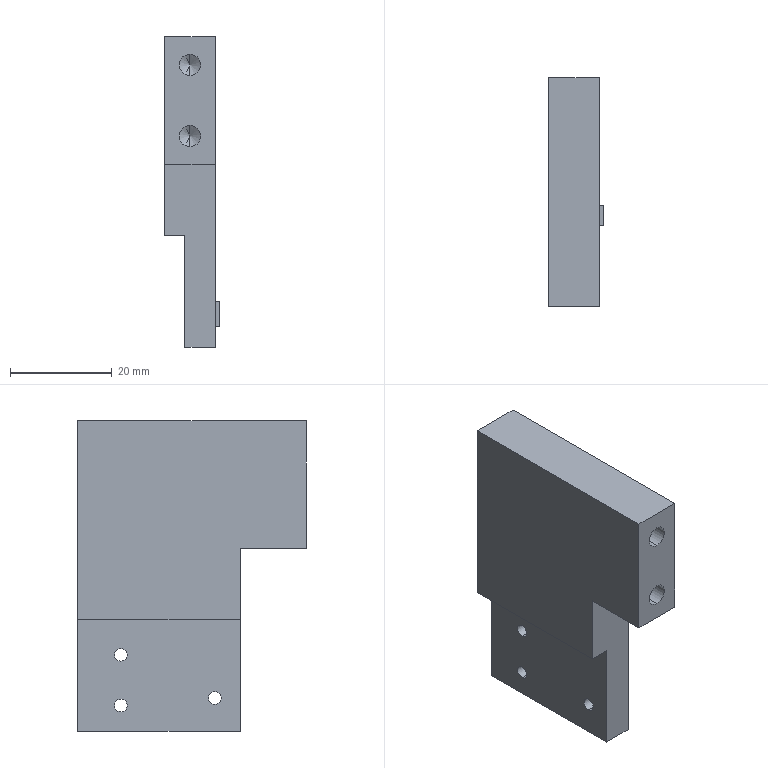Part | SolidWorks | features ICE 4, HoleWzd 3, ExtruThin 1 | 1 solid | 29 faces | box 10.8 x 45 x 61 mm | volume 19522 mm3 | plane 15 | cylinder 10 | cone 4 | commonest cylinder face diameters 2.5 x6 4.2 x4
STEP:
#1=CARTESIAN_POINT('',(10.8,18.,-30.75));
#2=VERTEX_POINT('',#1);
#3=CARTESIAN_POINT('',(10.8,18.,-28.25));
#4=VERTEX_POINT('',#3);
#5=CARTESIAN_POINT('',(10.8,18.,-29.5));
#6=DIRECTION('',(-1.,0.,0.));
#7=DIRECTION('',(0.,0.,1.));
#8=AXIS2_PLACEMENT_3D('',#5,#6,#7);
#9=CIRCLE('',#8,1.25);
#10=EDGE_CURVE('',#2,#4,#9,.T.);
#11=ORIENTED_EDGE('',*,*,#10,.F.);
#12=CARTESIAN_POINT('',(4.,18.,-30.75));
#13=VERTEX_POINT('',#12);
#14=CARTESIAN_POINT('',(0.,18.,-30.75));
#15=DIRECTION('',(-1.,0.,0.));
#16=VECTOR('',#15,1000.);
#17=LINE('',#14,#16);
#18=EDGE_CURVE('',#2,#13,#17,.T.);
#19=ORIENTED_EDGE('',*,*,#18,.T.);
#20=CARTESIAN_POINT('',(4.,18.,-28.25));
#21=VERTEX_POINT('',#20);
#22=CARTESIAN_POINT('',(4.,18.,-29.5));
#23=DIRECTION('',(1.,0.,0.));
#24=DIRECTION('',(0.,0.,-1.));
#25=AXIS2_PLACEMENT_3D('',#22,#23,#24);
#26=CIRCLE('',#25,1.25);
#27=EDGE_CURVE('',#21,#13,#26,.T.);
#28=ORIENTED_EDGE('',*,*,#27,.F.);
#29=CARTESIAN_POINT('',(0.,18.,-28.25));
#30=DIRECTION('',(-1.,0.,0.));
#31=VECTOR('',#30,1000.);
#32=LINE('',#29,#31);
#33=EDGE_CURVE('',#4,#21,#32,.T.);
#34=ORIENTED_EDGE('',*,*,#33,.F.);
#35=EDGE_LOOP('',(#11,#19,#28,#34));
#36=FACE_OUTER_BOUND('',#35,.T.);
#37=CARTESIAN_POINT('',(0.,18.,-29.5));
#38=DIRECTION('',(-1.,0.,0.));
#39=DIRECTION('',(0.,0.,1.));
#40=AXIS2_PLACEMENT_3D('',#37,#38,#39);
#41=CYLINDRICAL_SURFACE('',#40,1.25);
#42=ADVANCED_FACE('',(#36),#41,.F.);
#43=CARTESIAN_POINT('',(10.,36.5,-32.25));
#44=VERTEX_POINT('',#43);
#45=CARTESIAN_POINT('',(10.,36.5,-29.75));
#46=VERTEX_POINT('',#45);
#47=CARTESIAN_POINT('',(10.,36.5,-31.));
#48=DIRECTION('',(-1.,0.,0.));
#49=DIRECTION('',(0.,0.,1.));
#50=AXIS2_PLACEMENT_3D('',#47,#48,#49);
#51=CIRCLE('',#50,1.25);
#52=EDGE_CURVE('',#44,#46,#51,.T.);
#53=ORIENTED_EDGE('',*,*,#52,.F.);
#54=CARTESIAN_POINT('',(4.,36.5,-32.25));
#55=VERTEX_POINT('',#54);
#56=CARTESIAN_POINT('',(4.,36.5,-32.25));
#57=DIRECTION('',(-1.,0.,0.));
#58=VECTOR('',#57,1000.);
#59=LINE('',#56,#58);
#60=EDGE_CURVE('',#44,#55,#59,.T.);
#61=ORIENTED_EDGE('',*,*,#60,.T.);
#62=CARTESIAN_POINT('',(4.,36.5,-29.75));
#63=VERTEX_POINT('',#62);
#64=CARTESIAN_POINT('',(4.,36.5,-31.));
#65=DIRECTION('',(-1.,0.,0.));
#66=DIRECTION('',(0.,0.,1.));
#67=AXIS2_PLACEMENT_3D('',#64,#65,#66);
#68=CIRCLE('',#67,1.25);
#69=EDGE_CURVE('',#55,#63,#68,.T.);
#70=ORIENTED_EDGE('',*,*,#69,.T.);
#71=CARTESIAN_POINT('',(4.,36.5,-29.75));
#72=DIRECTION('',(-1.,0.,0.));
#73=VECTOR('',#72,1000.);
#74=LINE('',#71,#73);
#75=EDGE_CURVE('',#46,#63,#74,.T.);
#76=ORIENTED_EDGE('',*,*,#75,.F.);
#77=EDGE_LOOP('',(#53,#61,#70,#76));
#78=FACE_OUTER_BOUND('',#77,.T.);
#79=CARTESIAN_POINT('',(4.,36.5,-31.));
#80=DIRECTION('',(-1.,0.,0.));
#81=DIRECTION('',(0.,0.,1.));
#82=AXIS2_PLACEMENT_3D('',#79,#80,#81);
#83=CYLINDRICAL_SURFACE('',#82,1.25);
#84=ADVANCED_FACE('',(#78),#83,.F.);
#85=CARTESIAN_POINT('',(10.,36.5,-22.25));
#86=VERTEX_POINT('',#85);
#87=CARTESIAN_POINT('',(10.,36.5,-19.75));
#88=VERTEX_POINT('',#87);
#89=CARTESIAN_POINT('',(10.,36.5,-21.));
#90=DIRECTION('',(-1.,0.,0.));
#91=DIRECTION('',(0.,0.,1.));
#92=AXIS2_PLACEMENT_3D('',#89,#90,#91);
#93=CIRCLE('',#92,1.25);
#94=EDGE_CURVE('',#86,#88,#93,.T.);
#95=ORIENTED_EDGE('',*,*,#94,.F.);
#96=CARTESIAN_POINT('',(4.,36.5,-22.25));
#97=VERTEX_POINT('',#96);
#98=CARTESIAN_POINT('',(4.,36.5,-22.25));
#99=DIRECTION('',(-1.,0.,0.));
#100=VECTOR('',#99,1000.);
#101=LINE('',#98,#100);
#102=EDGE_CURVE('',#86,#97,#101,.T.);
#103=ORIENTED_EDGE('',*,*,#102,.T.);
#104=CARTESIAN_POINT('',(4.,36.5,-19.75));
#105=VERTEX_POINT('',#104);
#106=CARTESIAN_POINT('',(4.,36.5,-21.));
#107=DIRECTION('',(-1.,0.,0.));
#108=DIRECTION('',(0.,0.,1.));
#109=AXIS2_PLACEMENT_3D('',#106,#107,#108);
#110=CIRCLE('',#109,1.25);
#111=EDGE_CURVE('',#97,#105,#110,.T.);
#112=ORIENTED_EDGE('',*,*,#111,.T.);
#113=CARTESIAN_POINT('',(4.,36.5,-19.75));
#114=DIRECTION('',(-1.,0.,0.));
#115=VECTOR('',#114,1000.);
#116=LINE('',#113,#115);
#117=EDGE_CURVE('',#88,#105,#116,.T.);
#118=ORIENTED_EDGE('',*,*,#117,.F.);
#119=EDGE_LOOP('',(#95,#103,#112,#118));
#120=FACE_OUTER_BOUND('',#119,.T.);
#121=CARTESIAN_POINT('',(4.,36.5,-21.));
#122=DIRECTION('',(-1.,0.,0.));
#123=DIRECTION('',(0.,0.,1.));
#124=AXIS2_PLACEMENT_3D('',#121,#122,#123);
#125=CYLINDRICAL_SURFACE('',#124,1.25);
#126=ADVANCED_FACE('',(#120),#125,.F.);
#127=CARTESIAN_POINT('',(5.,12.4,7.6));
#128=VERTEX_POINT('',#127);
#129=CARTESIAN_POINT('',(5.,12.4,3.4));
#130=VERTEX_POINT('',#129);
#131=CARTESIAN_POINT('',(5.,12.4,5.5));
#132=DIRECTION('',(0.,-1.,0.));
#133=DIRECTION('',(0.,0.,-1.));
#134=AXIS2_PLACEMENT_3D('',#131,#132,#133);
#135=CIRCLE('',#134,2.1);
#136=EDGE_CURVE('',#128,#130,#135,.T.);
#137=ORIENTED_EDGE('',*,*,#136,.F.);
#138=CARTESIAN_POINT('',(5.,0.,7.6));
#139=VERTEX_POINT('',#138);
#140=CARTESIAN_POINT('',(5.,0.,7.6));
#141=DIRECTION('',(0.,-1.,0.));
#142=VECTOR('',#141,1000.);
#143=LINE('',#140,#142);
#144=EDGE_CURVE('',#128,#139,#143,.T.);
#145=ORIENTED_EDGE('',*,*,#144,.T.);
#146=CARTESIAN_POINT('',(5.,0.,3.4));
#147=VERTEX_POINT('',#146);
#148=CARTESIAN_POINT('',(5.,0.,5.5));
#149=DIRECTION('',(0.,-1.,0.));
#150=DIRECTION('',(0.,0.,-1.));
#151=AXIS2_PLACEMENT_3D('',#148,#149,#150);
#152=CIRCLE('',#151,2.1);
#153=EDGE_CURVE('',#139,#147,#152,.T.);
#154=ORIENTED_EDGE('',*,*,#153,.T.);
#155=CARTESIAN_POINT('',(5.,0.,3.4));
#156=DIRECTION('',(0.,-1.,0.));
#157=VECTOR('',#156,1000.);
#158=LINE('',#155,#157);
#159=EDGE_CURVE('',#130,#147,#158,.T.);
#160=ORIENTED_EDGE('',*,*,#159,.F.);
#161=EDGE_LOOP('',(#137,#145,#154,#160));
#162=FACE_OUTER_BOUND('',#161,.T.);
#163=CARTESIAN_POINT('',(5.,0.,5.5));
#164=DIRECTION('',(0.,-1.,0.));
#165=DIRECTION('',(0.,0.,-1.));
#166=AXIS2_PLACEMENT_3D('',#163,#164,#165);
#167=CYLINDRICAL_SURFACE('',#166,2.1);
#168=ADVANCED_FACE('',(#162),#167,.F.);
#169=CARTESIAN_POINT('',(5.,13.662,5.5));
#170=VERTEX_POINT('',#169);
#171=CARTESIAN_POINT('',(5.,12.4,3.4));
#172=DIRECTION('',(0.,-0.515,-0.8572));
#173=VECTOR('',#172,1000.);
#174=LINE('',#171,#173);
#175=EDGE_CURVE('',#170,#130,#174,.T.);
#176=ORIENTED_EDGE('',*,*,#175,.F.);
#177=CARTESIAN_POINT('',(5.,12.4,7.6));
#178=DIRECTION('',(0.,-0.515,0.8572));
#179=VECTOR('',#178,1000.);
#180=LINE('',#177,#179);
#181=EDGE_CURVE('',#170,#128,#180,.T.);
#182=ORIENTED_EDGE('',*,*,#181,.T.);
#183=ORIENTED_EDGE('',*,*,#136,.T.);
#184=EDGE_LOOP('',(#176,#182,#183));
#185=FACE_OUTER_BOUND('',#184,.T.);
#186=CARTESIAN_POINT('',(5.,12.4,5.5));
#187=DIRECTION('',(0.,-1.,0.));
#188=DIRECTION('',(0.,0.,-1.));
#189=AXIS2_PLACEMENT_3D('',#186,#187,#188);
#190=CONICAL_SURFACE('',#189,2.1,1.03);
#191=ADVANCED_FACE('',(#185),#190,.F.);
#192=CARTESIAN_POINT('',(5.,12.4,21.6));
#193=VERTEX_POINT('',#192);
#194=CARTESIAN_POINT('',(5.,12.4,17.4));
#195=VERTEX_POINT('',#194);
#196=CARTESIAN_POINT('',(5.,12.4,19.5));
#197=DIRECTION('',(0.,-1.,0.));
#198=DIRECTION('',(0.,0.,-1.));
#199=AXIS2_PLACEMENT_3D('',#196,#197,#198);
#200=CIRCLE('',#199,2.1);
#201=EDGE_CURVE('',#193,#195,#200,.T.);
#202=ORIENTED_EDGE('',*,*,#201,.F.);
#203=CARTESIAN_POINT('',(5.,0.,21.6));
#204=VERTEX_POINT('',#203);
#205=CARTESIAN_POINT('',(5.,0.,21.6));
#206=DIRECTION('',(0.,-1.,0.));
#207=VECTOR('',#206,1000.);
#208=LINE('',#205,#207);
#209=EDGE_CURVE('',#193,#204,#208,.T.);
#210=ORIENTED_EDGE('',*,*,#209,.T.);
#211=CARTESIAN_POINT('',(5.,0.,17.4));
#212=VERTEX_POINT('',#211);
#213=CARTESIAN_POINT('',(5.,0.,19.5));
#214=DIRECTION('',(0.,-1.,0.));
#215=DIRECTION('',(0.,0.,-1.));
#216=AXIS2_PLACEMENT_3D('',#213,#214,#215);
#217=CIRCLE('',#216,2.1);
#218=EDGE_CURVE('',#204,#212,#217,.T.);
#219=ORIENTED_EDGE('',*,*,#218,.T.);
#220=CARTESIAN_POINT('',(5.,0.,17.4));
#221=DIRECTION('',(0.,-1.,0.));
#222=VECTOR('',#221,1000.);
#223=LINE('',#220,#222);
#224=EDGE_CURVE('',#195,#212,#223,.T.);
#225=ORIENTED_EDGE('',*,*,#224,.F.);
#226=EDGE_LOOP('',(#202,#210,#219,#225));
#227=FACE_OUTER_BOUND('',#226,.T.);
#228=CARTESIAN_POINT('',(5.,0.,19.5));
#229=DIRECTION('',(0.,-1.,0.));
#230=DIRECTION('',(0.,0.,-1.));
#231=AXIS2_PLACEMENT_3D('',#228,#229,#230);
#232=CYLINDRICAL_SURFACE('',#231,2.1);
#233=ADVANCED_FACE('',(#227),#232,.F.);
#234=CARTESIAN_POINT('',(5.,13.662,19.5));
#235=VERTEX_POINT('',#234);
#236=CARTESIAN_POINT('',(5.,12.4,17.4));
#237=DIRECTION('',(0.,-0.515,-0.8572));
#238=VECTOR('',#237,1000.);
#239=LINE('',#236,#238);
#240=EDGE_CURVE('',#235,#195,#239,.T.);
#241=ORIENTED_EDGE('',*,*,#240,.F.);
#242=CARTESIAN_POINT('',(5.,12.4,21.6));
#243=DIRECTION('',(0.,-0.515,0.8572));
#244=VECTOR('',#243,1000.);
#245=LINE('',#242,#244);
#246=EDGE_CURVE('',#235,#193,#245,.T.);
#247=ORIENTED_EDGE('',*,*,#246,.T.);
#248=ORIENTED_EDGE('',*,*,#201,.T.);
#249=EDGE_LOOP('',(#241,#247,#248));
#250=FACE_OUTER_BOUND('',#249,.T.);
#251=CARTESIAN_POINT('',(5.,12.4,19.5));
#252=DIRECTION('',(0.,-1.,0.));
#253=DIRECTION('',(0.,0.,-1.));
#254=AXIS2_PLACEMENT_3D('',#251,#252,#253);
#255=CONICAL_SURFACE('',#254,2.1,1.03);
#256=ADVANCED_FACE('',(#250),#255,.F.);
#257=CARTESIAN_POINT('',(10.,0.,0.));
#258=VERTEX_POINT('',#257);
#259=CARTESIAN_POINT('',(10.,0.,25.));
#260=VERTEX_POINT('',#259);
#261=CARTESIAN_POINT('',(10.,0.,25.));
#262=DIRECTION('',(0.,0.,1.));
#263=VECTOR('',#262,1000.);
#264=LINE('',#261,#263);
#265=EDGE_CURVE('',#258,#260,#264,.T.);
#266=ORIENTED_EDGE('',*,*,#265,.F.);
#267=CARTESIAN_POINT('',(10.,13.,0.));
#268=VERTEX_POINT('',#267);
#269=CARTESIAN_POINT('',(10.,0.,0.));
#270=DIRECTION('',(0.,1.,0.));
#271=VECTOR('',#270,1000.);
#272=LINE('',#269,#271);
#273=EDGE_CURVE('',#258,#268,#272,.T.);
#274=ORIENTED_EDGE('',*,*,#273,.T.);
#275=CARTESIAN_POINT('',(10.,13.,-36.));
#276=VERTEX_POINT('',#275);
#277=CARTESIAN_POINT('',(10.,13.,0.));
#278=DIRECTION('',(0.,0.,-1.));
#279=VECTOR('',#278,1000.);
#280=LINE('',#277,#279);
#281=EDGE_CURVE('',#268,#276,#280,.T.);
#282=ORIENTED_EDGE('',*,*,#281,.T.);
#283=CARTESIAN_POINT('',(10.,45.,-36.));
#284=VERTEX_POINT('',#283);
#285=CARTESIAN_POINT('',(10.,45.,-36.));
#286=DIRECTION('',(0.,1.,0.));
#287=VECTOR('',#286,1000.);
#288=LINE('',#285,#287);
#289=EDGE_CURVE('',#276,#284,#288,.T.);
#290=ORIENTED_EDGE('',*,*,#289,.T.);
#291=CARTESIAN_POINT('',(10.,45.,25.));
#292=VERTEX_POINT('',#291);
#293=CARTESIAN_POINT('',(10.,45.,25.));
#294=DIRECTION('',(0.,0.,-1.));
#295=VECTOR('',#294,1000.);
#296=LINE('',#293,#295);
#297=EDGE_CURVE('',#292,#284,#296,.T.);
#298=ORIENTED_EDGE('',*,*,#297,.F.);
#299=CARTESIAN_POINT('',(10.,0.,25.));
#300=DIRECTION('',(0.,1.,0.));
#301=VECTOR('',#300,1000.);
#302=LINE('',#299,#301);
#303=EDGE_CURVE('',#260,#292,#302,.T.);
#304=ORIENTED_EDGE('',*,*,#303,.F.);
#305=EDGE_LOOP('',(#266,#274,#282,#290,#298,#304));
#306=FACE_OUTER_BOUND('',#305,.T.);
#307=CARTESIAN_POINT('',(10.,36.5,-21.));
#308=DIRECTION('',(-1.,0.,0.));
#309=DIRECTION('',(0.,0.,1.));
#310=AXIS2_PLACEMENT_3D('',#307,#308,#309);
#311=CIRCLE('',#310,1.25);
#312=EDGE_CURVE('',#88,#86,#311,.T.);
#313=ORIENTED_EDGE('',*,*,#312,.T.);
#314=ORIENTED_EDGE('',*,*,#94,.T.);
#315=EDGE_LOOP('',(#313,#314));
#316=FACE_BOUND('',#315,.T.);
#317=CARTESIAN_POINT('',(10.,36.5,-31.));
#318=DIRECTION('',(-1.,0.,0.));
#319=DIRECTION('',(0.,0.,1.));
#320=AXIS2_PLACEMENT_3D('',#317,#318,#319);
#321=CIRCLE('',#320,1.25);
#322=EDGE_CURVE('',#46,#44,#321,.T.);
#323=ORIENTED_EDGE('',*,*,#322,.T.);
#324=ORIENTED_EDGE('',*,*,#52,.T.);
#325=EDGE_LOOP('',(#323,#324));
#326=FACE_BOUND('',#325,.T.);
#327=CARTESIAN_POINT('',(10.,16.,-31.9));
#328=VERTEX_POINT('',#327);
#329=CARTESIAN_POINT('',(10.,20.,-31.9));
#330=VERTEX_POINT('',#329);
#331=CARTESIAN_POINT('',(10.,20.,-31.9));
#332=DIRECTION('',(0.,1.,0.));
#333=VECTOR('',#332,1000.);
#334=LINE('',#331,#333);
#335=EDGE_CURVE('',#328,#330,#334,.T.);
#336=ORIENTED_EDGE('',*,*,#335,.F.);
#337=CARTESIAN_POINT('',(10.,16.,-27.1));
#338=VERTEX_POINT('',#337);
#339=CARTESIAN_POINT('',(10.,16.,-27.1));
#340=DIRECTION('',(0.,0.,-1.));
#341=VECTOR('',#340,1000.);
#342=LINE('',#339,#341);
#343=EDGE_CURVE('',#338,#328,#342,.T.);
#344=ORIENTED_EDGE('',*,*,#343,.F.);
#345=CARTESIAN_POINT('',(10.,20.,-27.1));
#346=VERTEX_POINT('',#345);
#347=CARTESIAN_POINT('',(10.,20.,-27.1));
#348=DIRECTION('',(0.,-1.,0.));
#349=VECTOR('',#348,1000.);
#350=LINE('',#347,#349);
#351=EDGE_CURVE('',#346,#338,#350,.T.);
#352=ORIENTED_EDGE('',*,*,#351,.F.);
#353=CARTESIAN_POINT('',(10.,20.,-27.1));
#354=DIRECTION('',(0.,0.,1.));
#355=VECTOR('',#354,1000.);
#356=LINE('',#353,#355);
#357=EDGE_CURVE('',#330,#346,#356,.T.);
#358=ORIENTED_EDGE('',*,*,#357,.F.);
#359=EDGE_LOOP('',(#336,#344,#352,#358));
#360=FACE_BOUND('',#359,.T.);
#361=CARTESIAN_POINT('',(10.,0.,25.));
#362=DIRECTION('',(-1.,0.,0.));
#363=DIRECTION('',(0.,0.,1.));
#364=AXIS2_PLACEMENT_3D('',#361,#362,#363);
#365=PLANE('',#364);
#366=ADVANCED_FACE('',(#306,#316,#326,#360),#365,.F.);
#367=CARTESIAN_POINT('',(0.,0.,25.));
#368=VERTEX_POINT('',#367);
#369=CARTESIAN_POINT('',(0.,0.,25.));
#370=DIRECTION('',(-1.,0.,0.));
#371=VECTOR('',#370,1000.);
#372=LINE('',#369,#371);
#373=EDGE_CURVE('',#260,#368,#372,.T.);
#374=ORIENTED_EDGE('',*,*,#373,.F.);
#375=ORIENTED_EDGE('',*,*,#303,.T.);
#376=CARTESIAN_POINT('',(0.,45.,25.));
#377=VERTEX_POINT('',#376);
#378=CARTESIAN_POINT('',(0.,45.,25.));
#379=DIRECTION('',(1.,0.,0.));
#380=VECTOR('',#379,1000.);
#381=LINE('',#378,#380);
#382=EDGE_CURVE('',#377,#292,#381,.T.);
#383=ORIENTED_EDGE('',*,*,#382,.F.);
#384=CARTESIAN_POINT('',(0.,0.,25.));
#385=DIRECTION('',(0.,1.,0.));
#386=VECTOR('',#385,1000.);
#387=LINE('',#384,#386);
#388=EDGE_CURVE('',#368,#377,#387,.T.);
#389=ORIENTED_EDGE('',*,*,#388,.F.);
#390=EDGE_LOOP('',(#374,#375,#383,#389));
#391=FACE_OUTER_BOUND('',#390,.T.);
#392=CARTESIAN_POINT('',(0.,0.,25.));
#393=DIRECTION('',(0.,0.,-1.));
#394=DIRECTION('',(-1.,0.,0.));
#395=AXIS2_PLACEMENT_3D('',#392,#393,#394);
#396=PLANE('',#395);
#397=ADVANCED_FACE('',(#391),#396,.F.);
#398=ORIENTED_EDGE('',*,*,#273,.F.);
#399=CARTESIAN_POINT('',(0.,0.,0.));
#400=VERTEX_POINT('',#399);
#401=CARTESIAN_POINT('',(0.,0.,0.));
#402=DIRECTION('',(-1.,0.,0.));
#403=VECTOR('',#402,1000.);
#404=LINE('',#401,#403);
#405=EDGE_CURVE('',#258,#400,#404,.T.);
#406=ORIENTED_EDGE('',*,*,#405,.T.);
#407=CARTESIAN_POINT('',(0.,13.,0.));
#408=VERTEX_POINT('',#407);
#409=CARTESIAN_POINT('',(0.,0.,0.));
#410=DIRECTION('',(0.,1.,0.));
#411=VECTOR('',#410,1000.);
#412=LINE('',#409,#411);
#413=EDGE_CURVE('',#400,#408,#412,.T.);
#414=ORIENTED_EDGE('',*,*,#413,.T.);
#415=CARTESIAN_POINT('',(58.166,13.,0.));
#416=DIRECTION('',(-1.,0.,0.));
#417=VECTOR('',#416,1000.);
#418=LINE('',#415,#417);
#419=EDGE_CURVE('',#268,#408,#418,.T.);
#420=ORIENTED_EDGE('',*,*,#419,.F.);
#421=EDGE_LOOP('',(#398,#406,#414,#420));
#422=FACE_OUTER_BOUND('',#421,.T.);
#423=CARTESIAN_POINT('',(0.,0.,0.));
#424=DIRECTION('',(0.,0.,-1.));
#425=DIRECTION('',(-1.,0.,0.));
#426=AXIS2_PLACEMENT_3D('',#423,#424,#425);
#427=PLANE('',#426);
#428=ADVANCED_FACE('',(#422),#427,.T.);
#429=CARTESIAN_POINT('',(4.,45.,-14.));
#430=VERTEX_POINT('',#429);
#431=CARTESIAN_POINT('',(4.,45.,-36.));
#432=VERTEX_POINT('',#431);
#433=CARTESIAN_POINT('',(4.,45.,-36.));
#434=DIRECTION('',(0.,0.,-1.));
#435=VECTOR('',#434,1000.);
#436=LINE('',#433,#435);
#437=EDGE_CURVE('',#430,#432,#436,.T.);
#438=ORIENTED_EDGE('',*,*,#437,.F.);
#439=CARTESIAN_POINT('',(0.,45.,-14.));
#440=VERTEX_POINT('',#439);
#441=CARTESIAN_POINT('',(0.,45.,-14.));
#442=DIRECTION('',(1.,0.,0.));
#443=VECTOR('',#442,1000.);
#444=LINE('',#441,#443);
#445=EDGE_CURVE('',#440,#430,#444,.T.);
#446=ORIENTED_EDGE('',*,*,#445,.F.);
#447=CARTESIAN_POINT('',(0.,45.,25.));
#448=DIRECTION('',(0.,0.,-1.));
#449=VECTOR('',#448,1000.);
#450=LINE('',#447,#449);
#451=EDGE_CURVE('',#377,#440,#450,.T.);
#452=ORIENTED_EDGE('',*,*,#451,.F.);
#453=ORIENTED_EDGE('',*,*,#382,.T.);
#454=ORIENTED_EDGE('',*,*,#297,.T.);
#455=CARTESIAN_POINT('',(58.166,45.,-36.));
#456=DIRECTION('',(-1.,0.,0.));
#457=VECTOR('',#456,1000.);
#458=LINE('',#455,#457);
#459=EDGE_CURVE('',#284,#432,#458,.T.);
#460=ORIENTED_EDGE('',*,*,#459,.T.);
#461=EDGE_LOOP('',(#438,#446,#452,#453,#454,#460));
#462=FACE_OUTER_BOUND('',#461,.T.);
#463=CARTESIAN_POINT('',(0.,45.,25.));
#464=DIRECTION('',(0.,1.,0.));
#465=DIRECTION('',(0.,0.,1.));
#466=AXIS2_PLACEMENT_3D('',#463,#464,#465);
#467=PLANE('',#466);
#468=ADVANCED_FACE('',(#462),#467,.T.);
#469=CARTESIAN_POINT('',(0.,13.,-14.));
#470=VERTEX_POINT('',#469);
#471=CARTESIAN_POINT('',(0.,-10.,-14.));
#472=DIRECTION('',(0.,1.,0.));
#473=VECTOR('',#472,1000.);
#474=LINE('',#471,#473);
#475=EDGE_CURVE('',#470,#440,#474,.T.);
#476=ORIENTED_EDGE('',*,*,#475,.F.);
#477=CARTESIAN_POINT('',(0.,13.,0.));
#478=DIRECTION('',(0.,0.,1.));
#479=VECTOR('',#478,1000.);
#480=LINE('',#477,#479);
#481=EDGE_CURVE('',#470,#408,#480,.T.);
#482=ORIENTED_EDGE('',*,*,#481,.T.);
#483=ORIENTED_EDGE('',*,*,#413,.F.);
#484=CARTESIAN_POINT('',(0.,0.,25.));
#485=DIRECTION('',(0.,0.,-1.));
#486=VECTOR('',#485,1000.);
#487=LINE('',#484,#486);
#488=EDGE_CURVE('',#368,#400,#487,.T.);
#489=ORIENTED_EDGE('',*,*,#488,.F.);
#490=ORIENTED_EDGE('',*,*,#388,.T.);
#491=ORIENTED_EDGE('',*,*,#451,.T.);
#492=EDGE_LOOP('',(#476,#482,#483,#489,#490,#491));
#493=FACE_OUTER_BOUND('',#492,.T.);
#494=CARTESIAN_POINT('',(0.,0.,25.));
#495=DIRECTION('',(-1.,0.,0.));
#496=DIRECTION('',(0.,0.,1.));
#497=AXIS2_PLACEMENT_3D('',#494,#495,#496);
#498=PLANE('',#497);
#499=ADVANCED_FACE('',(#493),#498,.T.);
#500=CARTESIAN_POINT('',(4.,13.,-36.));
#501=VERTEX_POINT('',#500);
#502=CARTESIAN_POINT('',(4.,13.,-14.));
#503=VERTEX_POINT('',#502);
#504=CARTESIAN_POINT('',(4.,13.,0.));
#505=DIRECTION('',(0.,0.,1.));
#506=VECTOR('',#505,1000.);
#507=LINE('',#504,#506);
#508=EDGE_CURVE('',#501,#503,#507,.T.);
#509=ORIENTED_EDGE('',*,*,#508,.F.);
#510=CARTESIAN_POINT('',(58.166,13.,-36.));
#511=DIRECTION('',(-1.,0.,0.));
#512=VECTOR('',#511,1000.);
#513=LINE('',#510,#512);
#514=EDGE_CURVE('',#276,#501,#513,.T.);
#515=ORIENTED_EDGE('',*,*,#514,.F.);
#516=ORIENTED_EDGE('',*,*,#281,.F.);
#517=ORIENTED_EDGE('',*,*,#419,.T.);
#518=ORIENTED_EDGE('',*,*,#481,.F.);
#519=CARTESIAN_POINT('',(58.166,13.,-14.));
#520=DIRECTION('',(-1.,0.,0.));
#521=VECTOR('',#520,1000.);
#522=LINE('',#519,#521);
#523=EDGE_CURVE('',#503,#470,#522,.T.);
#524=ORIENTED_EDGE('',*,*,#523,.F.);
#525=EDGE_LOOP('',(#509,#515,#516,#517,#518,#524));
#526=FACE_OUTER_BOUND('',#525,.T.);
#527=CARTESIAN_POINT('',(58.166,13.,0.));
#528=DIRECTION('',(0.,-1.,0.));
#529=DIRECTION('',(0.,0.,-1.));
#530=AXIS2_PLACEMENT_3D('',#527,#528,#529);
#531=PLANE('',#530);
#532=ADVANCED_FACE('',(#526),#531,.T.);
#533=CARTESIAN_POINT('',(4.,45.,-36.));
#534=DIRECTION('',(0.,-1.,0.));
#535=VECTOR('',#534,1000.);
#536=LINE('',#533,#535);
#537=EDGE_CURVE('',#432,#501,#536,.T.);
#538=ORIENTED_EDGE('',*,*,#537,.F.);
#539=ORIENTED_EDGE('',*,*,#459,.F.);
#540=ORIENTED_EDGE('',*,*,#289,.F.);
#541=ORIENTED_EDGE('',*,*,#514,.T.);
#542=EDGE_LOOP('',(#538,#539,#540,#541));
#543=FACE_OUTER_BOUND('',#542,.T.);
#544=CARTESIAN_POINT('',(58.166,45.,-36.));
#545=DIRECTION('',(0.,0.,-1.));
#546=DIRECTION('',(-1.,0.,0.));
#547=AXIS2_PLACEMENT_3D('',#544,#545,#546);
#548=PLANE('',#547);
#549=ADVANCED_FACE('',(#543),#548,.T.);
#550=ORIENTED_EDGE('',*,*,#27,.T.);
#551=CARTESIAN_POINT('',(4.,18.,-29.5));
#552=DIRECTION('',(1.,0.,0.));
#553=DIRECTION('',(0.,0.,-1.));
#554=AXIS2_PLACEMENT_3D('',#551,#552,#553);
#555=CIRCLE('',#554,1.25);
#556=EDGE_CURVE('',#13,#21,#555,.T.);
#557=ORIENTED_EDGE('',*,*,#556,.T.);
#558=EDGE_LOOP('',(#550,#557));
#559=FACE_BOUND('',#558,.T.);
#560=CARTESIAN_POINT('',(4.,36.5,-31.));
#561=DIRECTION('',(-1.,0.,0.));
#562=DIRECTION('',(0.,0.,1.));
#563=AXIS2_PLACEMENT_3D('',#560,#561,#562);
#564=CIRCLE('',#563,1.25);
#565=EDGE_CURVE('',#63,#55,#564,.T.);
#566=ORIENTED_EDGE('',*,*,#565,.F.);
#567=ORIENTED_EDGE('',*,*,#69,.F.);
#568=EDGE_LOOP('',(#566,#567));
#569=FACE_BOUND('',#568,.T.);
#570=CARTESIAN_POINT('',(4.,36.5,-21.));
#571=DIRECTION('',(-1.,0.,0.));
#572=DIRECTION('',(0.,0.,1.));
#573=AXIS2_PLACEMENT_3D('',#570,#571,#572);
#574=CIRCLE('',#573,1.25);
#575=EDGE_CURVE('',#105,#97,#574,.T.);
#576=ORIENTED_EDGE('',*,*,#575,.F.);
#577=ORIENTED_EDGE('',*,*,#111,.F.);
#578=EDGE_LOOP('',(#576,#577));
#579=FACE_BOUND('',#578,.T.);
#580=ORIENTED_EDGE('',*,*,#508,.T.);
#581=CARTESIAN_POINT('',(4.,-10.,-14.));
#582=DIRECTION('',(0.,1.,0.));
#583=VECTOR('',#582,1000.);
#584=LINE('',#581,#583);
#585=EDGE_CURVE('',#503,#430,#584,.T.);
#586=ORIENTED_EDGE('',*,*,#585,.T.);
#587=ORIENTED_EDGE('',*,*,#437,.T.);
#588=ORIENTED_EDGE('',*,*,#537,.T.);
#589=EDGE_LOOP('',(#580,#586,#587,#588));
#590=FACE_OUTER_BOUND('',#589,.T.);
#591=CARTESIAN_POINT('',(4.,-10.,-36.));
#592=DIRECTION('',(1.,0.,0.));
#593=DIRECTION('',(0.,0.,-1.));
#594=AXIS2_PLACEMENT_3D('',#591,#592,#593);
#595=PLANE('',#594);
#596=ADVANCED_FACE('',(#559,#569,#579,#590),#595,.F.);
#597=ORIENTED_EDGE('',*,*,#523,.T.);
#598=ORIENTED_EDGE('',*,*,#475,.T.);
#599=ORIENTED_EDGE('',*,*,#445,.T.);
#600=ORIENTED_EDGE('',*,*,#585,.F.);
#601=EDGE_LOOP('',(#597,#598,#599,#600));
#602=FACE_OUTER_BOUND('',#601,.T.);
#603=CARTESIAN_POINT('',(0.,-10.,-14.));
#604=DIRECTION('',(0.,0.,1.));
#605=DIRECTION('',(1.,0.,0.));
#606=AXIS2_PLACEMENT_3D('',#603,#604,#605);
#607=PLANE('',#606);
#608=ADVANCED_FACE('',(#602),#607,.F.);
#609=CARTESIAN_POINT('',(5.,0.,5.5));
#610=DIRECTION('',(0.,-1.,0.));
#611=DIRECTION('',(0.,0.,-1.));
#612=AXIS2_PLACEMENT_3D('',#609,#610,#611);
#613=CIRCLE('',#612,2.1);
#614=EDGE_CURVE('',#147,#139,#613,.T.);
#615=ORIENTED_EDGE('',*,*,#614,.F.);
#616=ORIENTED_EDGE('',*,*,#153,.F.);
#617=EDGE_LOOP('',(#615,#616));
#618=FACE_BOUND('',#617,.T.);
#619=CARTESIAN_POINT('',(5.,0.,19.5));
#620=DIRECTION('',(0.,-1.,0.));
#621=DIRECTION('',(0.,0.,-1.));
#622=AXIS2_PLACEMENT_3D('',#619,#620,#621);
#623=CIRCLE('',#622,2.1);
#624=EDGE_CURVE('',#212,#204,#623,.T.);
#625=ORIENTED_EDGE('',*,*,#624,.F.);
#626=ORIENTED_EDGE('',*,*,#218,.F.);
#627=EDGE_LOOP('',(#625,#626));
#628=FACE_BOUND('',#627,.T.);
#629=ORIENTED_EDGE('',*,*,#405,.F.);
#630=ORIENTED_EDGE('',*,*,#265,.T.);
#631=ORIENTED_EDGE('',*,*,#373,.T.);
#632=ORIENTED_EDGE('',*,*,#488,.T.);
#633=EDGE_LOOP('',(#629,#630,#631,#632));
#634=FACE_OUTER_BOUND('',#633,.T.);
#635=CARTESIAN_POINT('',(0.,0.,0.));
#636=DIRECTION('',(0.,-1.,0.));
#637=DIRECTION('',(0.,0.,-1.));
#638=AXIS2_PLACEMENT_3D('',#635,#636,#637);
#639=PLANE('',#638);
#640=ADVANCED_FACE('',(#618,#628,#634),#639,.T.);
#641=ORIENTED_EDGE('',*,*,#246,.F.);
#642=ORIENTED_EDGE('',*,*,#240,.T.);
#643=CARTESIAN_POINT('',(5.,12.4,19.5));
#644=DIRECTION('',(0.,-1.,0.));
#645=DIRECTION('',(0.,0.,-1.));
#646=AXIS2_PLACEMENT_3D('',#643,#644,#645);
#647=CIRCLE('',#646,2.1);
#648=EDGE_CURVE('',#195,#193,#647,.T.);
#649=ORIENTED_EDGE('',*,*,#648,.T.);
#650=EDGE_LOOP('',(#641,#642,#649));
#651=FACE_OUTER_BOUND('',#650,.T.);
#652=CARTESIAN_POINT('',(5.,12.4,19.5));
#653=DIRECTION('',(0.,-1.,0.));
#654=DIRECTION('',(0.,0.,-1.));
#655=AXIS2_PLACEMENT_3D('',#652,#653,#654);
#656=CONICAL_SURFACE('',#655,2.1,1.03);
#657=ADVANCED_FACE('',(#651),#656,.F.);
#658=ORIENTED_EDGE('',*,*,#209,.F.);
#659=ORIENTED_EDGE('',*,*,#648,.F.);
#660=ORIENTED_EDGE('',*,*,#224,.T.);
#661=ORIENTED_EDGE('',*,*,#624,.T.);
#662=EDGE_LOOP('',(#658,#659,#660,#661));
#663=FACE_OUTER_BOUND('',#662,.T.);
#664=CARTESIAN_POINT('',(5.,0.,19.5));
#665=DIRECTION('',(0.,-1.,0.));
#666=DIRECTION('',(0.,0.,-1.));
#667=AXIS2_PLACEMENT_3D('',#664,#665,#666);
#668=CYLINDRICAL_SURFACE('',#667,2.1);
#669=ADVANCED_FACE('',(#663),#668,.F.);
#670=ORIENTED_EDGE('',*,*,#181,.F.);
#671=ORIENTED_EDGE('',*,*,#175,.T.);
#672=CARTESIAN_POINT('',(5.,12.4,5.5));
#673=DIRECTION('',(0.,-1.,0.));
#674=DIRECTION('',(0.,0.,-1.));
#675=AXIS2_PLACEMENT_3D('',#672,#673,#674);
#676=CIRCLE('',#675,2.1);
#677=EDGE_CURVE('',#130,#128,#676,.T.);
#678=ORIENTED_EDGE('',*,*,#677,.T.);
#679=EDGE_LOOP('',(#670,#671,#678));
#680=FACE_OUTER_BOUND('',#679,.T.);
#681=CARTESIAN_POINT('',(5.,12.4,5.5));
#682=DIRECTION('',(0.,-1.,0.));
#683=DIRECTION('',(0.,0.,-1.));
#684=AXIS2_PLACEMENT_3D('',#681,#682,#683);
#685=CONICAL_SURFACE('',#684,2.1,1.03);
#686=ADVANCED_FACE('',(#680),#685,.F.);
#687=ORIENTED_EDGE('',*,*,#144,.F.);
#688=ORIENTED_EDGE('',*,*,#677,.F.);
#689=ORIENTED_EDGE('',*,*,#159,.T.);
#690=ORIENTED_EDGE('',*,*,#614,.T.);
#691=EDGE_LOOP('',(#687,#688,#689,#690));
#692=FACE_OUTER_BOUND('',#691,.T.);
#693=CARTESIAN_POINT('',(5.,0.,5.5));
#694=DIRECTION('',(0.,-1.,0.));
#695=DIRECTION('',(0.,0.,-1.));
#696=AXIS2_PLACEMENT_3D('',#693,#694,#695);
#697=CYLINDRICAL_SURFACE('',#696,2.1);
#698=ADVANCED_FACE('',(#692),#697,.F.);
#699=ORIENTED_EDGE('',*,*,#102,.F.);
#700=ORIENTED_EDGE('',*,*,#312,.F.);
#701=ORIENTED_EDGE('',*,*,#117,.T.);
#702=ORIENTED_EDGE('',*,*,#575,.T.);
#703=EDGE_LOOP('',(#699,#700,#701,#702));
#704=FACE_OUTER_BOUND('',#703,.T.);
#705=CARTESIAN_POINT('',(4.,36.5,-21.));
#706=DIRECTION('',(-1.,0.,0.));
#707=DIRECTION('',(0.,0.,1.));
#708=AXIS2_PLACEMENT_3D('',#705,#706,#707);
#709=CYLINDRICAL_SURFACE('',#708,1.25);
#710=ADVANCED_FACE('',(#704),#709,.F.);
#711=ORIENTED_EDGE('',*,*,#60,.F.);
#712=ORIENTED_EDGE('',*,*,#322,.F.);
#713=ORIENTED_EDGE('',*,*,#75,.T.);
#714=ORIENTED_EDGE('',*,*,#565,.T.);
#715=EDGE_LOOP('',(#711,#712,#713,#714));
#716=FACE_OUTER_BOUND('',#715,.T.);
#717=CARTESIAN_POINT('',(4.,36.5,-31.));
#718=DIRECTION('',(-1.,0.,0.));
#719=DIRECTION('',(0.,0.,1.));
#720=AXIS2_PLACEMENT_3D('',#717,#718,#719);
#721=CYLINDRICAL_SURFACE('',#720,1.25);
#722=ADVANCED_FACE('',(#716),#721,.F.);
#723=ORIENTED_EDGE('',*,*,#335,.T.);
#724=CARTESIAN_POINT('',(10.8,20.,-31.9));
#725=VERTEX_POINT('',#724);
#726=CARTESIAN_POINT('',(10.8,20.,-31.9));
#727=DIRECTION('',(-1.,0.,0.));
#728=VECTOR('',#727,1000.);
#729=LINE('',#726,#728);
#730=EDGE_CURVE('',#725,#330,#729,.T.);
#731=ORIENTED_EDGE('',*,*,#730,.F.);
#732=CARTESIAN_POINT('',(10.8,16.,-31.9));
#733=VERTEX_POINT('',#732);
#734=CARTESIAN_POINT('',(10.8,20.,-31.9));
#735=DIRECTION('',(0.,1.,0.));
#736=VECTOR('',#735,1000.);
#737=LINE('',#734,#736);
#738=EDGE_CURVE('',#733,#725,#737,.T.);
#739=ORIENTED_EDGE('',*,*,#738,.F.);
#740=CARTESIAN_POINT('',(10.8,16.,-31.9));
#741=DIRECTION('',(-1.,0.,0.));
#742=VECTOR('',#741,1000.);
#743=LINE('',#740,#742);
#744=EDGE_CURVE('',#733,#328,#743,.T.);
#745=ORIENTED_EDGE('',*,*,#744,.T.);
#746=EDGE_LOOP('',(#723,#731,#739,#745));
#747=FACE_OUTER_BOUND('',#746,.T.);
#748=CARTESIAN_POINT('',(10.8,20.,-31.9));
#749=DIRECTION('',(0.,0.,1.));
#750=DIRECTION('',(1.,0.,0.));
#751=AXIS2_PLACEMENT_3D('',#748,#749,#750);
#752=PLANE('',#751);
#753=ADVANCED_FACE('',(#747),#752,.F.);
#754=ORIENTED_EDGE('',*,*,#357,.T.);
#755=CARTESIAN_POINT('',(10.8,20.,-27.1));
#756=VERTEX_POINT('',#755);
#757=CARTESIAN_POINT('',(10.8,20.,-27.1));
#758=DIRECTION('',(-1.,0.,0.));
#759=VECTOR('',#758,1000.);
#760=LINE('',#757,#759);
#761=EDGE_CURVE('',#756,#346,#760,.T.);
#762=ORIENTED_EDGE('',*,*,#761,.F.);
#763=CARTESIAN_POINT('',(10.8,20.,-27.1));
#764=DIRECTION('',(0.,0.,1.));
#765=VECTOR('',#764,1000.);
#766=LINE('',#763,#765);
#767=EDGE_CURVE('',#725,#756,#766,.T.);
#768=ORIENTED_EDGE('',*,*,#767,.F.);
#769=ORIENTED_EDGE('',*,*,#730,.T.);
#770=EDGE_LOOP('',(#754,#762,#768,#769));
#771=FACE_OUTER_BOUND('',#770,.T.);
#772=CARTESIAN_POINT('',(10.8,20.,-27.1));
#773=DIRECTION('',(0.,-1.,0.));
#774=DIRECTION('',(0.,0.,-1.));
#775=AXIS2_PLACEMENT_3D('',#772,#773,#774);
#776=PLANE('',#775);
#777=ADVANCED_FACE('',(#771),#776,.F.);
#778=ORIENTED_EDGE('',*,*,#351,.T.);
#779=CARTESIAN_POINT('',(10.8,16.,-27.1));
#780=VERTEX_POINT('',#779);
#781=CARTESIAN_POINT('',(10.8,16.,-27.1));
#782=DIRECTION('',(-1.,0.,0.));
#783=VECTOR('',#782,1000.);
#784=LINE('',#781,#783);
#785=EDGE_CURVE('',#780,#338,#784,.T.);
#786=ORIENTED_EDGE('',*,*,#785,.F.);
#787=CARTESIAN_POINT('',(10.8,20.,-27.1));
#788=DIRECTION('',(0.,-1.,0.));
#789=VECTOR('',#788,1000.);
#790=LINE('',#787,#789);
#791=EDGE_CURVE('',#756,#780,#790,.T.);
#792=ORIENTED_EDGE('',*,*,#791,.F.);
#793=ORIENTED_EDGE('',*,*,#761,.T.);
#794=EDGE_LOOP('',(#778,#786,#792,#793));
#795=FACE_OUTER_BOUND('',#794,.T.);
#796=CARTESIAN_POINT('',(10.8,20.,-27.1));
#797=DIRECTION('',(0.,0.,-1.));
#798=DIRECTION('',(-1.,0.,0.));
#799=AXIS2_PLACEMENT_3D('',#796,#797,#798);
#800=PLANE('',#799);
#801=ADVANCED_FACE('',(#795),#800,.F.);
#802=ORIENTED_EDGE('',*,*,#343,.T.);
#803=ORIENTED_EDGE('',*,*,#744,.F.);
#804=CARTESIAN_POINT('',(10.8,16.,-27.1));
#805=DIRECTION('',(0.,0.,-1.));
#806=VECTOR('',#805,1000.);
#807=LINE('',#804,#806);
#808=EDGE_CURVE('',#780,#733,#807,.T.);
#809=ORIENTED_EDGE('',*,*,#808,.F.);
#810=ORIENTED_EDGE('',*,*,#785,.T.);
#811=EDGE_LOOP('',(#802,#803,#809,#810));
#812=FACE_OUTER_BOUND('',#811,.T.);
#813=CARTESIAN_POINT('',(10.8,16.,-27.1));
#814=DIRECTION('',(0.,1.,0.));
#815=DIRECTION('',(0.,0.,1.));
#816=AXIS2_PLACEMENT_3D('',#813,#814,#815);
#817=PLANE('',#816);
#818=ADVANCED_FACE('',(#812),#817,.F.);
#819=CARTESIAN_POINT('',(10.8,18.,-29.5));
#820=DIRECTION('',(-1.,0.,0.));
#821=DIRECTION('',(0.,0.,1.));
#822=AXIS2_PLACEMENT_3D('',#819,#820,#821);
#823=CIRCLE('',#822,1.25);
#824=EDGE_CURVE('',#4,#2,#823,.T.);
#825=ORIENTED_EDGE('',*,*,#824,.T.);
#826=ORIENTED_EDGE('',*,*,#10,.T.);
#827=EDGE_LOOP('',(#825,#826));
#828=FACE_BOUND('',#827,.T.);
#829=ORIENTED_EDGE('',*,*,#738,.T.);
#830=ORIENTED_EDGE('',*,*,#767,.T.);
#831=ORIENTED_EDGE('',*,*,#791,.T.);
#832=ORIENTED_EDGE('',*,*,#808,.T.);
#833=EDGE_LOOP('',(#829,#830,#831,#832));
#834=FACE_OUTER_BOUND('',#833,.T.);
#835=CARTESIAN_POINT('',(10.8,0.,0.));
#836=DIRECTION('',(1.,0.,0.));
#837=DIRECTION('',(0.,0.,-1.));
#838=AXIS2_PLACEMENT_3D('',#835,#836,#837);
#839=PLANE('',#838);
#840=ADVANCED_FACE('',(#828,#834),#839,.T.);
#841=ORIENTED_EDGE('',*,*,#18,.F.);
#842=ORIENTED_EDGE('',*,*,#824,.F.);
#843=ORIENTED_EDGE('',*,*,#33,.T.);
#844=ORIENTED_EDGE('',*,*,#556,.F.);
#845=EDGE_LOOP('',(#841,#842,#843,#844));
#846=FACE_OUTER_BOUND('',#845,.T.);
#847=CARTESIAN_POINT('',(0.,18.,-29.5));
#848=DIRECTION('',(-1.,0.,0.));
#849=DIRECTION('',(0.,0.,1.));
#850=AXIS2_PLACEMENT_3D('',#847,#848,#849);
#851=CYLINDRICAL_SURFACE('',#850,1.25);
#852=ADVANCED_FACE('',(#846),#851,.F.);
#853=CLOSED_SHELL('',(#42,#84,#126,#168,#191,#233,#256,#366,#397,#428,#468,#499,#532,#549,#596,#608,#640,#657,#669,#686,#698,#710,#722,#753,#777,#801,#818,#840,#852));
#854=MANIFOLD_SOLID_BREP('',#853);
#855=CARTESIAN_POINT('',(0.,0.,0.));
#856=DIRECTION('',(0.,0.,1.));
#857=DIRECTION('',(1.,0.,0.));
#858=AXIS2_PLACEMENT_3D('',#855,#856,#857);
#859=(LENGTH_UNIT()NAMED_UNIT(*)SI_UNIT(.MILLI.,.METRE.));
#860=UNCERTAINTY_MEASURE_WITH_UNIT(LENGTH_MEASURE(0.00001),#859,'','');
#861=(NAMED_UNIT(*)PLANE_ANGLE_UNIT()SI_UNIT($,.RADIAN.));
#862=(NAMED_UNIT(*)SI_UNIT($,.STERADIAN.)SOLID_ANGLE_UNIT());
#863=(GEOMETRIC_REPRESENTATION_CONTEXT(3)GLOBAL_UNCERTAINTY_ASSIGNED_CONTEXT((#860))GLOBAL_UNIT_ASSIGNED_CONTEXT((#859,#861,#862))REPRESENTATION_CONTEXT('',''));
#864=ADVANCED_BREP_SHAPE_REPRESENTATION('',(#854,#858),#863);